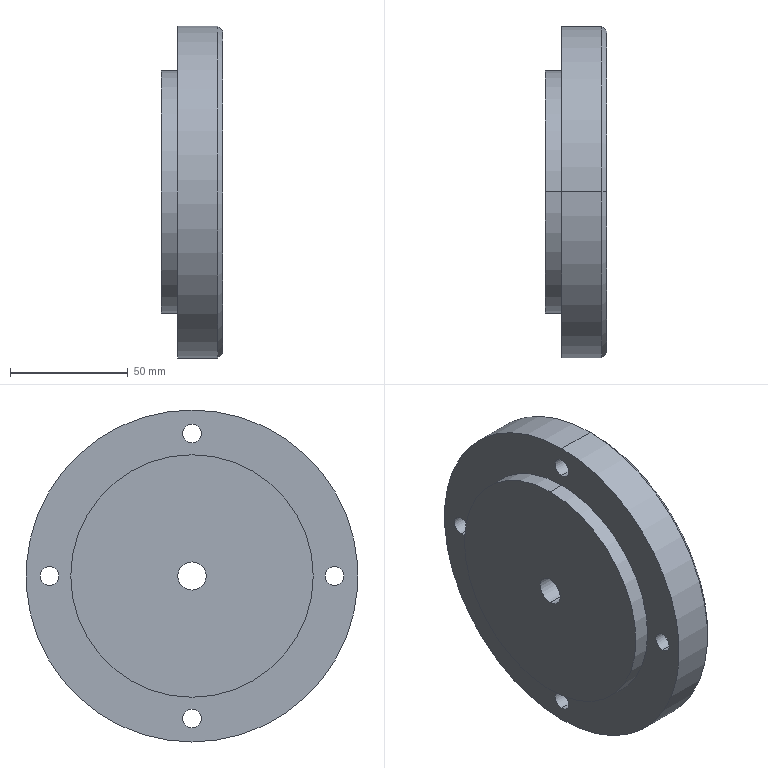Part | SolidWorks | features ICE 2, Chamfer 1, Revolution 1 | 1 solid | 34 faces | box 26 x 141 x 141 mm | volume 338840 mm3 | cylinder 22 | plane 8 | cone 4 | commonest cylinder face diameters 8 x8 14 x8 12 x2 103 x2 141 x2
STEP:
#1=CARTESIAN_POINT('',(-8.742,-60.5,7.));
#2=VERTEX_POINT('',#1);
#3=CARTESIAN_POINT('',(-8.742,-60.5,-7.));
#4=VERTEX_POINT('',#3);
#5=CARTESIAN_POINT('',(-8.742,-60.5,0.));
#6=DIRECTION('',(1.,0.,0.));
#7=DIRECTION('',(0.,0.,-1.));
#8=AXIS2_PLACEMENT_3D('',#5,#6,#7);
#9=CIRCLE('',#8,7.);
#10=EDGE_CURVE('',#2,#4,#9,.T.);
#11=ORIENTED_EDGE('',*,*,#10,.F.);
#12=CARTESIAN_POINT('',(-2.742,-60.5,7.));
#13=VERTEX_POINT('',#12);
#14=CARTESIAN_POINT('',(-8.742,-60.5,7.));
#15=DIRECTION('',(1.,0.,0.));
#16=VECTOR('',#15,1000.);
#17=LINE('',#14,#16);
#18=EDGE_CURVE('',#2,#13,#17,.T.);
#19=ORIENTED_EDGE('',*,*,#18,.T.);
#20=CARTESIAN_POINT('',(-2.742,-60.5,-7.));
#21=VERTEX_POINT('',#20);
#22=CARTESIAN_POINT('',(-2.742,-60.5,0.));
#23=DIRECTION('',(1.,0.,0.));
#24=DIRECTION('',(0.,0.,-1.));
#25=AXIS2_PLACEMENT_3D('',#22,#23,#24);
#26=CIRCLE('',#25,7.);
#27=EDGE_CURVE('',#13,#21,#26,.T.);
#28=ORIENTED_EDGE('',*,*,#27,.T.);
#29=CARTESIAN_POINT('',(-8.742,-60.5,-7.));
#30=DIRECTION('',(1.,0.,0.));
#31=VECTOR('',#30,1000.);
#32=LINE('',#29,#31);
#33=EDGE_CURVE('',#4,#21,#32,.T.);
#34=ORIENTED_EDGE('',*,*,#33,.F.);
#35=EDGE_LOOP('',(#11,#19,#28,#34));
#36=FACE_OUTER_BOUND('',#35,.T.);
#37=CARTESIAN_POINT('',(-8.742,-60.5,0.));
#38=DIRECTION('',(1.,0.,0.));
#39=DIRECTION('',(0.,0.,-1.));
#40=AXIS2_PLACEMENT_3D('',#37,#38,#39);
#41=CYLINDRICAL_SURFACE('',#40,7.);
#42=ADVANCED_FACE('',(#36),#41,.F.);
#43=CARTESIAN_POINT('',(-8.742,0.,-53.5));
#44=VERTEX_POINT('',#43);
#45=CARTESIAN_POINT('',(-8.742,0.,-67.5));
#46=VERTEX_POINT('',#45);
#47=CARTESIAN_POINT('',(-8.742,0.,-60.5));
#48=DIRECTION('',(1.,0.,0.));
#49=DIRECTION('',(0.,0.,-1.));
#50=AXIS2_PLACEMENT_3D('',#47,#48,#49);
#51=CIRCLE('',#50,7.);
#52=EDGE_CURVE('',#44,#46,#51,.T.);
#53=ORIENTED_EDGE('',*,*,#52,.F.);
#54=CARTESIAN_POINT('',(-2.742,0.,-53.5));
#55=VERTEX_POINT('',#54);
#56=CARTESIAN_POINT('',(-8.742,0.,-53.5));
#57=DIRECTION('',(1.,0.,0.));
#58=VECTOR('',#57,1000.);
#59=LINE('',#56,#58);
#60=EDGE_CURVE('',#44,#55,#59,.T.);
#61=ORIENTED_EDGE('',*,*,#60,.T.);
#62=CARTESIAN_POINT('',(-2.742,0.,-67.5));
#63=VERTEX_POINT('',#62);
#64=CARTESIAN_POINT('',(-2.742,0.,-60.5));
#65=DIRECTION('',(1.,0.,0.));
#66=DIRECTION('',(0.,0.,-1.));
#67=AXIS2_PLACEMENT_3D('',#64,#65,#66);
#68=CIRCLE('',#67,7.);
#69=EDGE_CURVE('',#55,#63,#68,.T.);
#70=ORIENTED_EDGE('',*,*,#69,.T.);
#71=CARTESIAN_POINT('',(-8.742,0.,-67.5));
#72=DIRECTION('',(1.,0.,0.));
#73=VECTOR('',#72,1000.);
#74=LINE('',#71,#73);
#75=EDGE_CURVE('',#46,#63,#74,.T.);
#76=ORIENTED_EDGE('',*,*,#75,.F.);
#77=EDGE_LOOP('',(#53,#61,#70,#76));
#78=FACE_OUTER_BOUND('',#77,.T.);
#79=CARTESIAN_POINT('',(-8.742,0.,-60.5));
#80=DIRECTION('',(1.,0.,0.));
#81=DIRECTION('',(0.,0.,-1.));
#82=AXIS2_PLACEMENT_3D('',#79,#80,#81);
#83=CYLINDRICAL_SURFACE('',#82,7.);
#84=ADVANCED_FACE('',(#78),#83,.F.);
#85=CARTESIAN_POINT('',(-8.742,60.5,7.));
#86=VERTEX_POINT('',#85);
#87=CARTESIAN_POINT('',(-8.742,60.5,-7.));
#88=VERTEX_POINT('',#87);
#89=CARTESIAN_POINT('',(-8.742,60.5,0.));
#90=DIRECTION('',(1.,0.,0.));
#91=DIRECTION('',(0.,0.,-1.));
#92=AXIS2_PLACEMENT_3D('',#89,#90,#91);
#93=CIRCLE('',#92,7.);
#94=EDGE_CURVE('',#86,#88,#93,.T.);
#95=ORIENTED_EDGE('',*,*,#94,.F.);
#96=CARTESIAN_POINT('',(-2.742,60.5,7.));
#97=VERTEX_POINT('',#96);
#98=CARTESIAN_POINT('',(-8.742,60.5,7.));
#99=DIRECTION('',(1.,0.,0.));
#100=VECTOR('',#99,1000.);
#101=LINE('',#98,#100);
#102=EDGE_CURVE('',#86,#97,#101,.T.);
#103=ORIENTED_EDGE('',*,*,#102,.T.);
#104=CARTESIAN_POINT('',(-2.742,60.5,-7.));
#105=VERTEX_POINT('',#104);
#106=CARTESIAN_POINT('',(-2.742,60.5,0.));
#107=DIRECTION('',(1.,0.,0.));
#108=DIRECTION('',(0.,0.,-1.));
#109=AXIS2_PLACEMENT_3D('',#106,#107,#108);
#110=CIRCLE('',#109,7.);
#111=EDGE_CURVE('',#97,#105,#110,.T.);
#112=ORIENTED_EDGE('',*,*,#111,.T.);
#113=CARTESIAN_POINT('',(-8.742,60.5,-7.));
#114=DIRECTION('',(1.,0.,0.));
#115=VECTOR('',#114,1000.);
#116=LINE('',#113,#115);
#117=EDGE_CURVE('',#88,#105,#116,.T.);
#118=ORIENTED_EDGE('',*,*,#117,.F.);
#119=EDGE_LOOP('',(#95,#103,#112,#118));
#120=FACE_OUTER_BOUND('',#119,.T.);
#121=CARTESIAN_POINT('',(-8.742,60.5,0.));
#122=DIRECTION('',(1.,0.,0.));
#123=DIRECTION('',(0.,0.,-1.));
#124=AXIS2_PLACEMENT_3D('',#121,#122,#123);
#125=CYLINDRICAL_SURFACE('',#124,7.);
#126=ADVANCED_FACE('',(#120),#125,.F.);
#127=CARTESIAN_POINT('',(-8.742,0.,67.5));
#128=VERTEX_POINT('',#127);
#129=CARTESIAN_POINT('',(-8.742,0.,53.5));
#130=VERTEX_POINT('',#129);
#131=CARTESIAN_POINT('',(-8.742,0.,60.5));
#132=DIRECTION('',(1.,0.,0.));
#133=DIRECTION('',(0.,0.,-1.));
#134=AXIS2_PLACEMENT_3D('',#131,#132,#133);
#135=CIRCLE('',#134,7.);
#136=EDGE_CURVE('',#128,#130,#135,.T.);
#137=ORIENTED_EDGE('',*,*,#136,.F.);
#138=CARTESIAN_POINT('',(-2.742,0.,67.5));
#139=VERTEX_POINT('',#138);
#140=CARTESIAN_POINT('',(-8.742,0.,67.5));
#141=DIRECTION('',(1.,0.,0.));
#142=VECTOR('',#141,1000.);
#143=LINE('',#140,#142);
#144=EDGE_CURVE('',#128,#139,#143,.T.);
#145=ORIENTED_EDGE('',*,*,#144,.T.);
#146=CARTESIAN_POINT('',(-2.742,0.,53.5));
#147=VERTEX_POINT('',#146);
#148=CARTESIAN_POINT('',(-2.742,0.,60.5));
#149=DIRECTION('',(1.,0.,0.));
#150=DIRECTION('',(0.,0.,-1.));
#151=AXIS2_PLACEMENT_3D('',#148,#149,#150);
#152=CIRCLE('',#151,7.);
#153=EDGE_CURVE('',#139,#147,#152,.T.);
#154=ORIENTED_EDGE('',*,*,#153,.T.);
#155=CARTESIAN_POINT('',(-8.742,0.,53.5));
#156=DIRECTION('',(1.,0.,0.));
#157=VECTOR('',#156,1000.);
#158=LINE('',#155,#157);
#159=EDGE_CURVE('',#130,#147,#158,.T.);
#160=ORIENTED_EDGE('',*,*,#159,.F.);
#161=EDGE_LOOP('',(#137,#145,#154,#160));
#162=FACE_OUTER_BOUND('',#161,.T.);
#163=CARTESIAN_POINT('',(-8.742,0.,60.5));
#164=DIRECTION('',(1.,0.,0.));
#165=DIRECTION('',(0.,0.,-1.));
#166=AXIS2_PLACEMENT_3D('',#163,#164,#165);
#167=CYLINDRICAL_SURFACE('',#166,7.);
#168=ADVANCED_FACE('',(#162),#167,.F.);
#169=CARTESIAN_POINT('',(-2.742,0.,-68.5));
#170=VERTEX_POINT('',#169);
#171=CARTESIAN_POINT('',(-2.742,0.,68.5));
#172=VERTEX_POINT('',#171);
#173=CARTESIAN_POINT('',(-2.742,0.,0.));
#174=DIRECTION('',(1.,0.,0.));
#175=DIRECTION('',(0.,0.,1.));
#176=AXIS2_PLACEMENT_3D('',#173,#174,#175);
#177=CIRCLE('',#176,68.5);
#178=EDGE_CURVE('',#170,#172,#177,.T.);
#179=ORIENTED_EDGE('',*,*,#178,.F.);
#180=CARTESIAN_POINT('',(-4.742,0.,-70.5));
#181=VERTEX_POINT('',#180);
#182=CARTESIAN_POINT('',(-4.742,0.,-70.5));
#183=DIRECTION('',(-0.7071,0.,-0.7071));
#184=VECTOR('',#183,1000.);
#185=LINE('',#182,#184);
#186=EDGE_CURVE('',#170,#181,#185,.T.);
#187=ORIENTED_EDGE('',*,*,#186,.T.);
#188=CARTESIAN_POINT('',(-4.742,0.,70.5));
#189=VERTEX_POINT('',#188);
#190=CARTESIAN_POINT('',(-4.742,0.,0.));
#191=DIRECTION('',(-1.,0.,0.));
#192=DIRECTION('',(0.,0.,1.));
#193=AXIS2_PLACEMENT_3D('',#190,#191,#192);
#194=CIRCLE('',#193,70.5);
#195=EDGE_CURVE('',#189,#181,#194,.T.);
#196=ORIENTED_EDGE('',*,*,#195,.F.);
#197=CARTESIAN_POINT('',(-4.742,0.,70.5));
#198=DIRECTION('',(-0.7071,0.,0.7071));
#199=VECTOR('',#198,1000.);
#200=LINE('',#197,#199);
#201=EDGE_CURVE('',#172,#189,#200,.T.);
#202=ORIENTED_EDGE('',*,*,#201,.F.);
#203=EDGE_LOOP('',(#179,#187,#196,#202));
#204=FACE_OUTER_BOUND('',#203,.T.);
#205=CARTESIAN_POINT('',(-4.742,0.,0.));
#206=DIRECTION('',(-1.,0.,0.));
#207=DIRECTION('',(0.,0.,1.));
#208=AXIS2_PLACEMENT_3D('',#205,#206,#207);
#209=CONICAL_SURFACE('',#208,70.5,0.7854);
#210=ADVANCED_FACE('',(#204),#209,.T.);
#211=CARTESIAN_POINT('',(-10.031,0.,-14.747));
#212=VERTEX_POINT('',#211);
#213=CARTESIAN_POINT('',(-10.031,0.,14.747));
#214=VERTEX_POINT('',#213);
#215=CARTESIAN_POINT('',(-10.031,0.,0.));
#216=DIRECTION('',(-1.,0.,0.));
#217=DIRECTION('',(0.,0.,1.));
#218=AXIS2_PLACEMENT_3D('',#215,#216,#217);
#219=CIRCLE('',#218,14.747);
#220=EDGE_CURVE('',#212,#214,#219,.T.);
#221=ORIENTED_EDGE('',*,*,#220,.T.);
#222=CARTESIAN_POINT('',(-2.742,0.,19.746));
#223=VERTEX_POINT('',#222);
#224=CARTESIAN_POINT('',(-10.031,0.,14.747));
#225=DIRECTION('',(0.8247,0.,0.5655));
#226=VECTOR('',#225,1000.);
#227=LINE('',#224,#226);
#228=EDGE_CURVE('',#214,#223,#227,.T.);
#229=ORIENTED_EDGE('',*,*,#228,.T.);
#230=CARTESIAN_POINT('',(-2.742,0.,-19.746));
#231=VERTEX_POINT('',#230);
#232=CARTESIAN_POINT('',(-2.742,0.,0.));
#233=DIRECTION('',(-1.,0.,0.));
#234=DIRECTION('',(0.,0.,1.));
#235=AXIS2_PLACEMENT_3D('',#232,#233,#234);
#236=CIRCLE('',#235,19.746);
#237=EDGE_CURVE('',#231,#223,#236,.T.);
#238=ORIENTED_EDGE('',*,*,#237,.F.);
#239=CARTESIAN_POINT('',(-10.031,0.,-14.747));
#240=DIRECTION('',(0.8247,0.,-0.5655));
#241=VECTOR('',#240,1000.);
#242=LINE('',#239,#241);
#243=EDGE_CURVE('',#212,#231,#242,.T.);
#244=ORIENTED_EDGE('',*,*,#243,.F.);
#245=EDGE_LOOP('',(#221,#229,#238,#244));
#246=FACE_OUTER_BOUND('',#245,.T.);
#247=CARTESIAN_POINT('',(-10.031,0.,0.));
#248=DIRECTION('',(1.,0.,0.));
#249=DIRECTION('',(0.,0.,-1.));
#250=AXIS2_PLACEMENT_3D('',#247,#248,#249);
#251=CONICAL_SURFACE('',#250,14.747,0.6011);
#252=ADVANCED_FACE('',(#246),#251,.F.);
#253=ORIENTED_EDGE('',*,*,#195,.T.);
#254=CARTESIAN_POINT('',(-21.742,0.,-70.5));
#255=VERTEX_POINT('',#254);
#256=CARTESIAN_POINT('',(-75.394,0.,-70.5));
#257=DIRECTION('',(-1.,0.,0.));
#258=VECTOR('',#257,1000.);
#259=LINE('',#256,#258);
#260=EDGE_CURVE('',#181,#255,#259,.T.);
#261=ORIENTED_EDGE('',*,*,#260,.T.);
#262=CARTESIAN_POINT('',(-21.742,0.,70.5));
#263=VERTEX_POINT('',#262);
#264=CARTESIAN_POINT('',(-21.742,0.,0.));
#265=DIRECTION('',(-1.,0.,0.));
#266=DIRECTION('',(0.,0.,1.));
#267=AXIS2_PLACEMENT_3D('',#264,#265,#266);
#268=CIRCLE('',#267,70.5);
#269=EDGE_CURVE('',#263,#255,#268,.T.);
#270=ORIENTED_EDGE('',*,*,#269,.F.);
#271=CARTESIAN_POINT('',(-75.394,0.,70.5));
#272=DIRECTION('',(-1.,0.,0.));
#273=VECTOR('',#272,1000.);
#274=LINE('',#271,#273);
#275=EDGE_CURVE('',#189,#263,#274,.T.);
#276=ORIENTED_EDGE('',*,*,#275,.F.);
#277=EDGE_LOOP('',(#253,#261,#270,#276));
#278=FACE_OUTER_BOUND('',#277,.T.);
#279=CARTESIAN_POINT('',(-75.394,0.,0.));
#280=DIRECTION('',(-1.,0.,0.));
#281=DIRECTION('',(0.,0.,1.));
#282=AXIS2_PLACEMENT_3D('',#279,#280,#281);
#283=CYLINDRICAL_SURFACE('',#282,70.5);
#284=ADVANCED_FACE('',(#278),#283,.T.);
#285=CARTESIAN_POINT('',(-21.742,0.,51.5));
#286=VERTEX_POINT('',#285);
#287=CARTESIAN_POINT('',(-21.742,0.,-51.5));
#288=VERTEX_POINT('',#287);
#289=CARTESIAN_POINT('',(-21.742,0.,0.));
#290=DIRECTION('',(-1.,0.,0.));
#291=DIRECTION('',(0.,0.,1.));
#292=AXIS2_PLACEMENT_3D('',#289,#290,#291);
#293=CIRCLE('',#292,51.5);
#294=EDGE_CURVE('',#286,#288,#293,.T.);
#295=ORIENTED_EDGE('',*,*,#294,.T.);
#296=CARTESIAN_POINT('',(-28.742,0.,-51.5));
#297=VERTEX_POINT('',#296);
#298=CARTESIAN_POINT('',(-75.394,0.,-51.5));
#299=DIRECTION('',(-1.,0.,0.));
#300=VECTOR('',#299,1000.);
#301=LINE('',#298,#300);
#302=EDGE_CURVE('',#288,#297,#301,.T.);
#303=ORIENTED_EDGE('',*,*,#302,.T.);
#304=CARTESIAN_POINT('',(-28.742,0.,51.5));
#305=VERTEX_POINT('',#304);
#306=CARTESIAN_POINT('',(-28.742,0.,0.));
#307=DIRECTION('',(-1.,0.,0.));
#308=DIRECTION('',(0.,0.,1.));
#309=AXIS2_PLACEMENT_3D('',#306,#307,#308);
#310=CIRCLE('',#309,51.5);
#311=EDGE_CURVE('',#305,#297,#310,.T.);
#312=ORIENTED_EDGE('',*,*,#311,.F.);
#313=CARTESIAN_POINT('',(-75.394,0.,51.5));
#314=DIRECTION('',(-1.,0.,0.));
#315=VECTOR('',#314,1000.);
#316=LINE('',#313,#315);
#317=EDGE_CURVE('',#286,#305,#316,.T.);
#318=ORIENTED_EDGE('',*,*,#317,.F.);
#319=EDGE_LOOP('',(#295,#303,#312,#318));
#320=FACE_OUTER_BOUND('',#319,.T.);
#321=CARTESIAN_POINT('',(-75.394,0.,0.));
#322=DIRECTION('',(-1.,0.,0.));
#323=DIRECTION('',(0.,0.,1.));
#324=AXIS2_PLACEMENT_3D('',#321,#322,#323);
#325=CYLINDRICAL_SURFACE('',#324,51.5);
#326=ADVANCED_FACE('',(#320),#325,.T.);
#327=CARTESIAN_POINT('',(-10.031,0.,-6.));
#328=VERTEX_POINT('',#327);
#329=CARTESIAN_POINT('',(-10.031,0.,6.));
#330=VERTEX_POINT('',#329);
#331=CARTESIAN_POINT('',(-10.031,0.,0.));
#332=DIRECTION('',(-1.,0.,0.));
#333=DIRECTION('',(0.,0.,1.));
#334=AXIS2_PLACEMENT_3D('',#331,#332,#333);
#335=CIRCLE('',#334,6.);
#336=EDGE_CURVE('',#328,#330,#335,.T.);
#337=ORIENTED_EDGE('',*,*,#336,.F.);
#338=CARTESIAN_POINT('',(-28.742,0.,-6.));
#339=VERTEX_POINT('',#338);
#340=CARTESIAN_POINT('',(-75.394,0.,-6.));
#341=DIRECTION('',(-1.,0.,0.));
#342=VECTOR('',#341,1000.);
#343=LINE('',#340,#342);
#344=EDGE_CURVE('',#328,#339,#343,.T.);
#345=ORIENTED_EDGE('',*,*,#344,.T.);
#346=CARTESIAN_POINT('',(-28.742,0.,6.));
#347=VERTEX_POINT('',#346);
#348=CARTESIAN_POINT('',(-28.742,0.,0.));
#349=DIRECTION('',(-1.,0.,0.));
#350=DIRECTION('',(0.,0.,1.));
#351=AXIS2_PLACEMENT_3D('',#348,#349,#350);
#352=CIRCLE('',#351,6.);
#353=EDGE_CURVE('',#339,#347,#352,.T.);
#354=ORIENTED_EDGE('',*,*,#353,.T.);
#355=CARTESIAN_POINT('',(-75.394,0.,6.));
#356=DIRECTION('',(-1.,0.,0.));
#357=VECTOR('',#356,1000.);
#358=LINE('',#355,#357);
#359=EDGE_CURVE('',#330,#347,#358,.T.);
#360=ORIENTED_EDGE('',*,*,#359,.F.);
#361=EDGE_LOOP('',(#337,#345,#354,#360));
#362=FACE_OUTER_BOUND('',#361,.T.);
#363=CARTESIAN_POINT('',(-75.394,0.,0.));
#364=DIRECTION('',(-1.,0.,0.));
#365=DIRECTION('',(0.,0.,1.));
#366=AXIS2_PLACEMENT_3D('',#363,#364,#365);
#367=CYLINDRICAL_SURFACE('',#366,6.);
#368=ADVANCED_FACE('',(#362),#367,.F.);
#369=CARTESIAN_POINT('',(-21.742,0.,64.5));
#370=VERTEX_POINT('',#369);
#371=CARTESIAN_POINT('',(-21.742,0.,56.5));
#372=VERTEX_POINT('',#371);
#373=CARTESIAN_POINT('',(-21.742,0.,60.5));
#374=DIRECTION('',(1.,0.,0.));
#375=DIRECTION('',(0.,0.,-1.));
#376=AXIS2_PLACEMENT_3D('',#373,#374,#375);
#377=CIRCLE('',#376,4.);
#378=EDGE_CURVE('',#370,#372,#377,.T.);
#379=ORIENTED_EDGE('',*,*,#378,.F.);
#380=CARTESIAN_POINT('',(-8.742,0.,64.5));
#381=VERTEX_POINT('',#380);
#382=CARTESIAN_POINT('',(-51.742,0.,64.5));
#383=DIRECTION('',(1.,0.,0.));
#384=VECTOR('',#383,1000.);
#385=LINE('',#382,#384);
#386=EDGE_CURVE('',#370,#381,#385,.T.);
#387=ORIENTED_EDGE('',*,*,#386,.T.);
#388=CARTESIAN_POINT('',(-8.742,0.,56.5));
#389=VERTEX_POINT('',#388);
#390=CARTESIAN_POINT('',(-8.742,0.,60.5));
#391=DIRECTION('',(-1.,0.,0.));
#392=DIRECTION('',(0.,0.,-1.));
#393=AXIS2_PLACEMENT_3D('',#390,#391,#392);
#394=CIRCLE('',#393,4.);
#395=EDGE_CURVE('',#389,#381,#394,.T.);
#396=ORIENTED_EDGE('',*,*,#395,.F.);
#397=CARTESIAN_POINT('',(-51.742,0.,56.5));
#398=DIRECTION('',(1.,0.,0.));
#399=VECTOR('',#398,1000.);
#400=LINE('',#397,#399);
#401=EDGE_CURVE('',#372,#389,#400,.T.);
#402=ORIENTED_EDGE('',*,*,#401,.F.);
#403=EDGE_LOOP('',(#379,#387,#396,#402));
#404=FACE_OUTER_BOUND('',#403,.T.);
#405=CARTESIAN_POINT('',(-51.742,0.,60.5));
#406=DIRECTION('',(1.,0.,0.));
#407=DIRECTION('',(0.,0.,-1.));
#408=AXIS2_PLACEMENT_3D('',#405,#406,#407);
#409=CYLINDRICAL_SURFACE('',#408,4.);
#410=ADVANCED_FACE('',(#404),#409,.F.);
#411=CARTESIAN_POINT('',(-21.742,60.5,4.));
#412=VERTEX_POINT('',#411);
#413=CARTESIAN_POINT('',(-21.742,60.5,-4.));
#414=VERTEX_POINT('',#413);
#415=CARTESIAN_POINT('',(-21.742,60.5,0.));
#416=DIRECTION('',(1.,0.,0.));
#417=DIRECTION('',(0.,0.,-1.));
#418=AXIS2_PLACEMENT_3D('',#415,#416,#417);
#419=CIRCLE('',#418,4.);
#420=EDGE_CURVE('',#412,#414,#419,.T.);
#421=ORIENTED_EDGE('',*,*,#420,.F.);
#422=CARTESIAN_POINT('',(-8.742,60.5,4.));
#423=VERTEX_POINT('',#422);
#424=CARTESIAN_POINT('',(-51.742,60.5,4.));
#425=DIRECTION('',(1.,0.,0.));
#426=VECTOR('',#425,1000.);
#427=LINE('',#424,#426);
#428=EDGE_CURVE('',#412,#423,#427,.T.);
#429=ORIENTED_EDGE('',*,*,#428,.T.);
#430=CARTESIAN_POINT('',(-8.742,60.5,-4.));
#431=VERTEX_POINT('',#430);
#432=CARTESIAN_POINT('',(-8.742,60.5,0.));
#433=DIRECTION('',(-1.,0.,0.));
#434=DIRECTION('',(0.,0.,-1.));
#435=AXIS2_PLACEMENT_3D('',#432,#433,#434);
#436=CIRCLE('',#435,4.);
#437=EDGE_CURVE('',#431,#423,#436,.T.);
#438=ORIENTED_EDGE('',*,*,#437,.F.);
#439=CARTESIAN_POINT('',(-51.742,60.5,-4.));
#440=DIRECTION('',(1.,0.,0.));
#441=VECTOR('',#440,1000.);
#442=LINE('',#439,#441);
#443=EDGE_CURVE('',#414,#431,#442,.T.);
#444=ORIENTED_EDGE('',*,*,#443,.F.);
#445=EDGE_LOOP('',(#421,#429,#438,#444));
#446=FACE_OUTER_BOUND('',#445,.T.);
#447=CARTESIAN_POINT('',(-51.742,60.5,0.));
#448=DIRECTION('',(1.,0.,0.));
#449=DIRECTION('',(0.,0.,-1.));
#450=AXIS2_PLACEMENT_3D('',#447,#448,#449);
#451=CYLINDRICAL_SURFACE('',#450,4.);
#452=ADVANCED_FACE('',(#446),#451,.F.);
#453=CARTESIAN_POINT('',(-21.742,0.,-56.5));
#454=VERTEX_POINT('',#453);
#455=CARTESIAN_POINT('',(-21.742,0.,-64.5));
#456=VERTEX_POINT('',#455);
#457=CARTESIAN_POINT('',(-21.742,0.,-60.5));
#458=DIRECTION('',(1.,0.,0.));
#459=DIRECTION('',(0.,0.,-1.));
#460=AXIS2_PLACEMENT_3D('',#457,#458,#459);
#461=CIRCLE('',#460,4.);
#462=EDGE_CURVE('',#454,#456,#461,.T.);
#463=ORIENTED_EDGE('',*,*,#462,.F.);
#464=CARTESIAN_POINT('',(-8.742,0.,-56.5));
#465=VERTEX_POINT('',#464);
#466=CARTESIAN_POINT('',(-51.742,0.,-56.5));
#467=DIRECTION('',(1.,0.,0.));
#468=VECTOR('',#467,1000.);
#469=LINE('',#466,#468);
#470=EDGE_CURVE('',#454,#465,#469,.T.);
#471=ORIENTED_EDGE('',*,*,#470,.T.);
#472=CARTESIAN_POINT('',(-8.742,0.,-64.5));
#473=VERTEX_POINT('',#472);
#474=CARTESIAN_POINT('',(-8.742,0.,-60.5));
#475=DIRECTION('',(-1.,0.,0.));
#476=DIRECTION('',(0.,0.,-1.));
#477=AXIS2_PLACEMENT_3D('',#474,#475,#476);
#478=CIRCLE('',#477,4.);
#479=EDGE_CURVE('',#473,#465,#478,.T.);
#480=ORIENTED_EDGE('',*,*,#479,.F.);
#481=CARTESIAN_POINT('',(-51.742,0.,-64.5));
#482=DIRECTION('',(1.,0.,0.));
#483=VECTOR('',#482,1000.);
#484=LINE('',#481,#483);
#485=EDGE_CURVE('',#456,#473,#484,.T.);
#486=ORIENTED_EDGE('',*,*,#485,.F.);
#487=EDGE_LOOP('',(#463,#471,#480,#486));
#488=FACE_OUTER_BOUND('',#487,.T.);
#489=CARTESIAN_POINT('',(-51.742,0.,-60.5));
#490=DIRECTION('',(1.,0.,0.));
#491=DIRECTION('',(0.,0.,-1.));
#492=AXIS2_PLACEMENT_3D('',#489,#490,#491);
#493=CYLINDRICAL_SURFACE('',#492,4.);
#494=ADVANCED_FACE('',(#488),#493,.F.);
#495=CARTESIAN_POINT('',(-21.742,-60.5,4.));
#496=VERTEX_POINT('',#495);
#497=CARTESIAN_POINT('',(-21.742,-60.5,-4.));
#498=VERTEX_POINT('',#497);
#499=CARTESIAN_POINT('',(-21.742,-60.5,0.));
#500=DIRECTION('',(1.,0.,0.));
#501=DIRECTION('',(0.,0.,-1.));
#502=AXIS2_PLACEMENT_3D('',#499,#500,#501);
#503=CIRCLE('',#502,4.);
#504=EDGE_CURVE('',#496,#498,#503,.T.);
#505=ORIENTED_EDGE('',*,*,#504,.F.);
#506=CARTESIAN_POINT('',(-8.742,-60.5,4.));
#507=VERTEX_POINT('',#506);
#508=CARTESIAN_POINT('',(-51.742,-60.5,4.));
#509=DIRECTION('',(1.,0.,0.));
#510=VECTOR('',#509,1000.);
#511=LINE('',#508,#510);
#512=EDGE_CURVE('',#496,#507,#511,.T.);
#513=ORIENTED_EDGE('',*,*,#512,.T.);
#514=CARTESIAN_POINT('',(-8.742,-60.5,-4.));
#515=VERTEX_POINT('',#514);
#516=CARTESIAN_POINT('',(-8.742,-60.5,0.));
#517=DIRECTION('',(-1.,0.,0.));
#518=DIRECTION('',(0.,0.,-1.));
#519=AXIS2_PLACEMENT_3D('',#516,#517,#518);
#520=CIRCLE('',#519,4.);
#521=EDGE_CURVE('',#515,#507,#520,.T.);
#522=ORIENTED_EDGE('',*,*,#521,.F.);
#523=CARTESIAN_POINT('',(-51.742,-60.5,-4.));
#524=DIRECTION('',(1.,0.,0.));
#525=VECTOR('',#524,1000.);
#526=LINE('',#523,#525);
#527=EDGE_CURVE('',#498,#515,#526,.T.);
#528=ORIENTED_EDGE('',*,*,#527,.F.);
#529=EDGE_LOOP('',(#505,#513,#522,#528));
#530=FACE_OUTER_BOUND('',#529,.T.);
#531=CARTESIAN_POINT('',(-51.742,-60.5,0.));
#532=DIRECTION('',(1.,0.,0.));
#533=DIRECTION('',(0.,0.,-1.));
#534=AXIS2_PLACEMENT_3D('',#531,#532,#533);
#535=CYLINDRICAL_SURFACE('',#534,4.);
#536=ADVANCED_FACE('',(#530),#535,.F.);
#537=ORIENTED_EDGE('',*,*,#512,.F.);
#538=CARTESIAN_POINT('',(-21.742,-60.5,0.));
#539=DIRECTION('',(1.,0.,0.));
#540=DIRECTION('',(0.,0.,-1.));
#541=AXIS2_PLACEMENT_3D('',#538,#539,#540);
#542=CIRCLE('',#541,4.);
#543=EDGE_CURVE('',#498,#496,#542,.T.);
#544=ORIENTED_EDGE('',*,*,#543,.F.);
#545=ORIENTED_EDGE('',*,*,#527,.T.);
#546=CARTESIAN_POINT('',(-8.742,-60.5,0.));
#547=DIRECTION('',(-1.,0.,0.));
#548=DIRECTION('',(0.,0.,-1.));
#549=AXIS2_PLACEMENT_3D('',#546,#547,#548);
#550=CIRCLE('',#549,4.);
#551=EDGE_CURVE('',#507,#515,#550,.T.);
#552=ORIENTED_EDGE('',*,*,#551,.F.);
#553=EDGE_LOOP('',(#537,#544,#545,#552));
#554=FACE_OUTER_BOUND('',#553,.T.);
#555=CARTESIAN_POINT('',(-51.742,-60.5,0.));
#556=DIRECTION('',(1.,0.,0.));
#557=DIRECTION('',(0.,0.,-1.));
#558=AXIS2_PLACEMENT_3D('',#555,#556,#557);
#559=CYLINDRICAL_SURFACE('',#558,4.);
#560=ADVANCED_FACE('',(#554),#559,.F.);
#561=ORIENTED_EDGE('',*,*,#470,.F.);
#562=CARTESIAN_POINT('',(-21.742,0.,-60.5));
#563=DIRECTION('',(1.,0.,0.));
#564=DIRECTION('',(0.,0.,-1.));
#565=AXIS2_PLACEMENT_3D('',#562,#563,#564);
#566=CIRCLE('',#565,4.);
#567=EDGE_CURVE('',#456,#454,#566,.T.);
#568=ORIENTED_EDGE('',*,*,#567,.F.);
#569=ORIENTED_EDGE('',*,*,#485,.T.);
#570=CARTESIAN_POINT('',(-8.742,0.,-60.5));
#571=DIRECTION('',(-1.,0.,0.));
#572=DIRECTION('',(0.,0.,-1.));
#573=AXIS2_PLACEMENT_3D('',#570,#571,#572);
#574=CIRCLE('',#573,4.);
#575=EDGE_CURVE('',#465,#473,#574,.T.);
#576=ORIENTED_EDGE('',*,*,#575,.F.);
#577=EDGE_LOOP('',(#561,#568,#569,#576));
#578=FACE_OUTER_BOUND('',#577,.T.);
#579=CARTESIAN_POINT('',(-51.742,0.,-60.5));
#580=DIRECTION('',(1.,0.,0.));
#581=DIRECTION('',(0.,0.,-1.));
#582=AXIS2_PLACEMENT_3D('',#579,#580,#581);
#583=CYLINDRICAL_SURFACE('',#582,4.);
#584=ADVANCED_FACE('',(#578),#583,.F.);
#585=ORIENTED_EDGE('',*,*,#428,.F.);
#586=CARTESIAN_POINT('',(-21.742,60.5,0.));
#587=DIRECTION('',(1.,0.,0.));
#588=DIRECTION('',(0.,0.,-1.));
#589=AXIS2_PLACEMENT_3D('',#586,#587,#588);
#590=CIRCLE('',#589,4.);
#591=EDGE_CURVE('',#414,#412,#590,.T.);
#592=ORIENTED_EDGE('',*,*,#591,.F.);
#593=ORIENTED_EDGE('',*,*,#443,.T.);
#594=CARTESIAN_POINT('',(-8.742,60.5,0.));
#595=DIRECTION('',(-1.,0.,0.));
#596=DIRECTION('',(0.,0.,-1.));
#597=AXIS2_PLACEMENT_3D('',#594,#595,#596);
#598=CIRCLE('',#597,4.);
#599=EDGE_CURVE('',#423,#431,#598,.T.);
#600=ORIENTED_EDGE('',*,*,#599,.F.);
#601=EDGE_LOOP('',(#585,#592,#593,#600));
#602=FACE_OUTER_BOUND('',#601,.T.);
#603=CARTESIAN_POINT('',(-51.742,60.5,0.));
#604=DIRECTION('',(1.,0.,0.));
#605=DIRECTION('',(0.,0.,-1.));
#606=AXIS2_PLACEMENT_3D('',#603,#604,#605);
#607=CYLINDRICAL_SURFACE('',#606,4.);
#608=ADVANCED_FACE('',(#602),#607,.F.);
#609=ORIENTED_EDGE('',*,*,#386,.F.);
#610=CARTESIAN_POINT('',(-21.742,0.,60.5));
#611=DIRECTION('',(1.,0.,0.));
#612=DIRECTION('',(0.,0.,-1.));
#613=AXIS2_PLACEMENT_3D('',#610,#611,#612);
#614=CIRCLE('',#613,4.);
#615=EDGE_CURVE('',#372,#370,#614,.T.);
#616=ORIENTED_EDGE('',*,*,#615,.F.);
#617=ORIENTED_EDGE('',*,*,#401,.T.);
#618=CARTESIAN_POINT('',(-8.742,0.,60.5));
#619=DIRECTION('',(-1.,0.,0.));
#620=DIRECTION('',(0.,0.,-1.));
#621=AXIS2_PLACEMENT_3D('',#618,#619,#620);
#622=CIRCLE('',#621,4.);
#623=EDGE_CURVE('',#381,#389,#622,.T.);
#624=ORIENTED_EDGE('',*,*,#623,.F.);
#625=EDGE_LOOP('',(#609,#616,#617,#624));
#626=FACE_OUTER_BOUND('',#625,.T.);
#627=CARTESIAN_POINT('',(-51.742,0.,60.5));
#628=DIRECTION('',(1.,0.,0.));
#629=DIRECTION('',(0.,0.,-1.));
#630=AXIS2_PLACEMENT_3D('',#627,#628,#629);
#631=CYLINDRICAL_SURFACE('',#630,4.);
#632=ADVANCED_FACE('',(#626),#631,.F.);
#633=ORIENTED_EDGE('',*,*,#344,.F.);
#634=CARTESIAN_POINT('',(-10.031,0.,0.));
#635=DIRECTION('',(-1.,0.,0.));
#636=DIRECTION('',(0.,0.,1.));
#637=AXIS2_PLACEMENT_3D('',#634,#635,#636);
#638=CIRCLE('',#637,6.);
#639=EDGE_CURVE('',#330,#328,#638,.T.);
#640=ORIENTED_EDGE('',*,*,#639,.F.);
#641=ORIENTED_EDGE('',*,*,#359,.T.);
#642=CARTESIAN_POINT('',(-28.742,0.,0.));
#643=DIRECTION('',(-1.,0.,0.));
#644=DIRECTION('',(0.,0.,1.));
#645=AXIS2_PLACEMENT_3D('',#642,#643,#644);
#646=CIRCLE('',#645,6.);
#647=EDGE_CURVE('',#347,#339,#646,.T.);
#648=ORIENTED_EDGE('',*,*,#647,.T.);
#649=EDGE_LOOP('',(#633,#640,#641,#648));
#650=FACE_OUTER_BOUND('',#649,.T.);
#651=CARTESIAN_POINT('',(-75.394,0.,0.));
#652=DIRECTION('',(-1.,0.,0.));
#653=DIRECTION('',(0.,0.,1.));
#654=AXIS2_PLACEMENT_3D('',#651,#652,#653);
#655=CYLINDRICAL_SURFACE('',#654,6.);
#656=ADVANCED_FACE('',(#650),#655,.F.);
#657=ORIENTED_EDGE('',*,*,#647,.F.);
#658=ORIENTED_EDGE('',*,*,#353,.F.);
#659=EDGE_LOOP('',(#657,#658));
#660=FACE_BOUND('',#659,.T.);
#661=ORIENTED_EDGE('',*,*,#311,.T.);
#662=CARTESIAN_POINT('',(-28.742,0.,0.));
#663=DIRECTION('',(-1.,0.,0.));
#664=DIRECTION('',(0.,0.,1.));
#665=AXIS2_PLACEMENT_3D('',#662,#663,#664);
#666=CIRCLE('',#665,51.5);
#667=EDGE_CURVE('',#297,#305,#666,.T.);
#668=ORIENTED_EDGE('',*,*,#667,.T.);
#669=EDGE_LOOP('',(#661,#668));
#670=FACE_OUTER_BOUND('',#669,.T.);
#671=CARTESIAN_POINT('',(-28.742,6.,0.));
#672=DIRECTION('',(1.,0.,0.));
#673=DIRECTION('',(0.,0.,-1.));
#674=AXIS2_PLACEMENT_3D('',#671,#672,#673);
#675=PLANE('',#674);
#676=ADVANCED_FACE('',(#660,#670),#675,.F.);
#677=ORIENTED_EDGE('',*,*,#302,.F.);
#678=CARTESIAN_POINT('',(-21.742,0.,0.));
#679=DIRECTION('',(-1.,0.,0.));
#680=DIRECTION('',(0.,0.,1.));
#681=AXIS2_PLACEMENT_3D('',#678,#679,#680);
#682=CIRCLE('',#681,51.5);
#683=EDGE_CURVE('',#288,#286,#682,.T.);
#684=ORIENTED_EDGE('',*,*,#683,.T.);
#685=ORIENTED_EDGE('',*,*,#317,.T.);
#686=ORIENTED_EDGE('',*,*,#667,.F.);
#687=EDGE_LOOP('',(#677,#684,#685,#686));
#688=FACE_OUTER_BOUND('',#687,.T.);
#689=CARTESIAN_POINT('',(-75.394,0.,0.));
#690=DIRECTION('',(-1.,0.,0.));
#691=DIRECTION('',(0.,0.,1.));
#692=AXIS2_PLACEMENT_3D('',#689,#690,#691);
#693=CYLINDRICAL_SURFACE('',#692,51.5);
#694=ADVANCED_FACE('',(#688),#693,.T.);
#695=ORIENTED_EDGE('',*,*,#615,.T.);
#696=ORIENTED_EDGE('',*,*,#378,.T.);
#697=EDGE_LOOP('',(#695,#696));
#698=FACE_BOUND('',#697,.T.);
#699=ORIENTED_EDGE('',*,*,#591,.T.);
#700=ORIENTED_EDGE('',*,*,#420,.T.);
#701=EDGE_LOOP('',(#699,#700));
#702=FACE_BOUND('',#701,.T.);
#703=ORIENTED_EDGE('',*,*,#567,.T.);
#704=ORIENTED_EDGE('',*,*,#462,.T.);
#705=EDGE_LOOP('',(#703,#704));
#706=FACE_BOUND('',#705,.T.);
#707=ORIENTED_EDGE('',*,*,#543,.T.);
#708=ORIENTED_EDGE('',*,*,#504,.T.);
#709=EDGE_LOOP('',(#707,#708));
#710=FACE_BOUND('',#709,.T.);
#711=ORIENTED_EDGE('',*,*,#294,.F.);
#712=ORIENTED_EDGE('',*,*,#683,.F.);
#713=EDGE_LOOP('',(#711,#712));
#714=FACE_BOUND('',#713,.T.);
#715=ORIENTED_EDGE('',*,*,#269,.T.);
#716=CARTESIAN_POINT('',(-21.742,0.,0.));
#717=DIRECTION('',(-1.,0.,0.));
#718=DIRECTION('',(0.,0.,1.));
#719=AXIS2_PLACEMENT_3D('',#716,#717,#718);
#720=CIRCLE('',#719,70.5);
#721=EDGE_CURVE('',#255,#263,#720,.T.);
#722=ORIENTED_EDGE('',*,*,#721,.T.);
#723=EDGE_LOOP('',(#715,#722));
#724=FACE_OUTER_BOUND('',#723,.T.);
#725=CARTESIAN_POINT('',(-21.742,51.5,0.));
#726=DIRECTION('',(1.,0.,0.));
#727=DIRECTION('',(0.,0.,-1.));
#728=AXIS2_PLACEMENT_3D('',#725,#726,#727);
#729=PLANE('',#728);
#730=ADVANCED_FACE('',(#698,#702,#706,#710,#714,#724),#729,.F.);
#731=ORIENTED_EDGE('',*,*,#260,.F.);
#732=CARTESIAN_POINT('',(-4.742,0.,0.));
#733=DIRECTION('',(-1.,0.,0.));
#734=DIRECTION('',(0.,0.,1.));
#735=AXIS2_PLACEMENT_3D('',#732,#733,#734);
#736=CIRCLE('',#735,70.5);
#737=EDGE_CURVE('',#181,#189,#736,.T.);
#738=ORIENTED_EDGE('',*,*,#737,.T.);
#739=ORIENTED_EDGE('',*,*,#275,.T.);
#740=ORIENTED_EDGE('',*,*,#721,.F.);
#741=EDGE_LOOP('',(#731,#738,#739,#740));
#742=FACE_OUTER_BOUND('',#741,.T.);
#743=CARTESIAN_POINT('',(-75.394,0.,0.));
#744=DIRECTION('',(-1.,0.,0.));
#745=DIRECTION('',(0.,0.,1.));
#746=AXIS2_PLACEMENT_3D('',#743,#744,#745);
#747=CYLINDRICAL_SURFACE('',#746,70.5);
#748=ADVANCED_FACE('',(#742),#747,.T.);
#749=CARTESIAN_POINT('',(-2.742,60.5,0.));
#750=DIRECTION('',(1.,0.,0.));
#751=DIRECTION('',(0.,0.,-1.));
#752=AXIS2_PLACEMENT_3D('',#749,#750,#751);
#753=CIRCLE('',#752,7.);
#754=EDGE_CURVE('',#105,#97,#753,.T.);
#755=ORIENTED_EDGE('',*,*,#754,.F.);
#756=ORIENTED_EDGE('',*,*,#111,.F.);
#757=EDGE_LOOP('',(#755,#756));
#758=FACE_BOUND('',#757,.T.);
#759=CARTESIAN_POINT('',(-2.742,0.,-60.5));
#760=DIRECTION('',(1.,0.,0.));
#761=DIRECTION('',(0.,0.,-1.));
#762=AXIS2_PLACEMENT_3D('',#759,#760,#761);
#763=CIRCLE('',#762,7.);
#764=EDGE_CURVE('',#63,#55,#763,.T.);
#765=ORIENTED_EDGE('',*,*,#764,.F.);
#766=ORIENTED_EDGE('',*,*,#69,.F.);
#767=EDGE_LOOP('',(#765,#766));
#768=FACE_BOUND('',#767,.T.);
#769=CARTESIAN_POINT('',(-2.742,-60.5,0.));
#770=DIRECTION('',(1.,0.,0.));
#771=DIRECTION('',(0.,0.,-1.));
#772=AXIS2_PLACEMENT_3D('',#769,#770,#771);
#773=CIRCLE('',#772,7.);
#774=EDGE_CURVE('',#21,#13,#773,.T.);
#775=ORIENTED_EDGE('',*,*,#774,.F.);
#776=ORIENTED_EDGE('',*,*,#27,.F.);
#777=EDGE_LOOP('',(#775,#776));
#778=FACE_BOUND('',#777,.T.);
#779=CARTESIAN_POINT('',(-2.742,0.,60.5));
#780=DIRECTION('',(1.,0.,0.));
#781=DIRECTION('',(0.,0.,-1.));
#782=AXIS2_PLACEMENT_3D('',#779,#780,#781);
#783=CIRCLE('',#782,7.);
#784=EDGE_CURVE('',#147,#139,#783,.T.);
#785=ORIENTED_EDGE('',*,*,#784,.F.);
#786=ORIENTED_EDGE('',*,*,#153,.F.);
#787=EDGE_LOOP('',(#785,#786));
#788=FACE_BOUND('',#787,.T.);
#789=CARTESIAN_POINT('',(-2.742,0.,0.));
#790=DIRECTION('',(1.,0.,0.));
#791=DIRECTION('',(0.,0.,1.));
#792=AXIS2_PLACEMENT_3D('',#789,#790,#791);
#793=CIRCLE('',#792,68.5);
#794=EDGE_CURVE('',#172,#170,#793,.T.);
#795=ORIENTED_EDGE('',*,*,#794,.T.);
#796=ORIENTED_EDGE('',*,*,#178,.T.);
#797=EDGE_LOOP('',(#795,#796));
#798=FACE_OUTER_BOUND('',#797,.T.);
#799=ORIENTED_EDGE('',*,*,#237,.T.);
#800=CARTESIAN_POINT('',(-2.742,0.,0.));
#801=DIRECTION('',(-1.,0.,0.));
#802=DIRECTION('',(0.,0.,1.));
#803=AXIS2_PLACEMENT_3D('',#800,#801,#802);
#804=CIRCLE('',#803,19.746);
#805=EDGE_CURVE('',#223,#231,#804,.T.);
#806=ORIENTED_EDGE('',*,*,#805,.T.);
#807=EDGE_LOOP('',(#799,#806));
#808=FACE_BOUND('',#807,.T.);
#809=CARTESIAN_POINT('',(-2.742,70.5,0.));
#810=DIRECTION('',(-1.,0.,0.));
#811=DIRECTION('',(0.,0.,1.));
#812=AXIS2_PLACEMENT_3D('',#809,#810,#811);
#813=PLANE('',#812);
#814=ADVANCED_FACE('',(#758,#768,#778,#788,#798,#808),#813,.F.);
#815=ORIENTED_EDGE('',*,*,#228,.F.);
#816=CARTESIAN_POINT('',(-10.031,0.,0.));
#817=DIRECTION('',(-1.,0.,0.));
#818=DIRECTION('',(0.,0.,1.));
#819=AXIS2_PLACEMENT_3D('',#816,#817,#818);
#820=CIRCLE('',#819,14.747);
#821=EDGE_CURVE('',#214,#212,#820,.T.);
#822=ORIENTED_EDGE('',*,*,#821,.T.);
#823=ORIENTED_EDGE('',*,*,#243,.T.);
#824=ORIENTED_EDGE('',*,*,#805,.F.);
#825=EDGE_LOOP('',(#815,#822,#823,#824));
#826=FACE_OUTER_BOUND('',#825,.T.);
#827=CARTESIAN_POINT('',(-10.031,0.,0.));
#828=DIRECTION('',(1.,0.,0.));
#829=DIRECTION('',(0.,0.,-1.));
#830=AXIS2_PLACEMENT_3D('',#827,#828,#829);
#831=CONICAL_SURFACE('',#830,14.747,0.6011);
#832=ADVANCED_FACE('',(#826),#831,.F.);
#833=ORIENTED_EDGE('',*,*,#220,.F.);
#834=ORIENTED_EDGE('',*,*,#821,.F.);
#835=EDGE_LOOP('',(#833,#834));
#836=FACE_OUTER_BOUND('',#835,.T.);
#837=ORIENTED_EDGE('',*,*,#639,.T.);
#838=ORIENTED_EDGE('',*,*,#336,.T.);
#839=EDGE_LOOP('',(#837,#838));
#840=FACE_BOUND('',#839,.T.);
#841=CARTESIAN_POINT('',(-10.031,14.747,0.));
#842=DIRECTION('',(-1.,0.,0.));
#843=DIRECTION('',(0.,0.,1.));
#844=AXIS2_PLACEMENT_3D('',#841,#842,#843);
#845=PLANE('',#844);
#846=ADVANCED_FACE('',(#836,#840),#845,.F.);
#847=ORIENTED_EDGE('',*,*,#186,.F.);
#848=ORIENTED_EDGE('',*,*,#794,.F.);
#849=ORIENTED_EDGE('',*,*,#201,.T.);
#850=ORIENTED_EDGE('',*,*,#737,.F.);
#851=EDGE_LOOP('',(#847,#848,#849,#850));
#852=FACE_OUTER_BOUND('',#851,.T.);
#853=CARTESIAN_POINT('',(-4.742,0.,0.));
#854=DIRECTION('',(-1.,0.,0.));
#855=DIRECTION('',(0.,0.,1.));
#856=AXIS2_PLACEMENT_3D('',#853,#854,#855);
#857=CONICAL_SURFACE('',#856,70.5,0.7854);
#858=ADVANCED_FACE('',(#852),#857,.T.);
#859=CARTESIAN_POINT('',(-8.742,0.,60.5));
#860=DIRECTION('',(1.,0.,0.));
#861=DIRECTION('',(0.,0.,-1.));
#862=AXIS2_PLACEMENT_3D('',#859,#860,#861);
#863=CIRCLE('',#862,7.);
#864=EDGE_CURVE('',#130,#128,#863,.T.);
#865=ORIENTED_EDGE('',*,*,#864,.T.);
#866=ORIENTED_EDGE('',*,*,#136,.T.);
#867=EDGE_LOOP('',(#865,#866));
#868=FACE_OUTER_BOUND('',#867,.T.);
#869=ORIENTED_EDGE('',*,*,#395,.T.);
#870=ORIENTED_EDGE('',*,*,#623,.T.);
#871=EDGE_LOOP('',(#869,#870));
#872=FACE_BOUND('',#871,.T.);
#873=CARTESIAN_POINT('',(-8.742,0.,60.5));
#874=DIRECTION('',(1.,0.,0.));
#875=DIRECTION('',(0.,0.,-1.));
#876=AXIS2_PLACEMENT_3D('',#873,#874,#875);
#877=PLANE('',#876);
#878=ADVANCED_FACE('',(#868,#872),#877,.T.);
#879=ORIENTED_EDGE('',*,*,#144,.F.);
#880=ORIENTED_EDGE('',*,*,#864,.F.);
#881=ORIENTED_EDGE('',*,*,#159,.T.);
#882=ORIENTED_EDGE('',*,*,#784,.T.);
#883=EDGE_LOOP('',(#879,#880,#881,#882));
#884=FACE_OUTER_BOUND('',#883,.T.);
#885=CARTESIAN_POINT('',(-8.742,0.,60.5));
#886=DIRECTION('',(1.,0.,0.));
#887=DIRECTION('',(0.,0.,-1.));
#888=AXIS2_PLACEMENT_3D('',#885,#886,#887);
#889=CYLINDRICAL_SURFACE('',#888,7.);
#890=ADVANCED_FACE('',(#884),#889,.F.);
#891=CARTESIAN_POINT('',(-8.742,60.5,0.));
#892=DIRECTION('',(1.,0.,0.));
#893=DIRECTION('',(0.,0.,-1.));
#894=AXIS2_PLACEMENT_3D('',#891,#892,#893);
#895=CIRCLE('',#894,7.);
#896=EDGE_CURVE('',#88,#86,#895,.T.);
#897=ORIENTED_EDGE('',*,*,#896,.T.);
#898=ORIENTED_EDGE('',*,*,#94,.T.);
#899=EDGE_LOOP('',(#897,#898));
#900=FACE_OUTER_BOUND('',#899,.T.);
#901=ORIENTED_EDGE('',*,*,#437,.T.);
#902=ORIENTED_EDGE('',*,*,#599,.T.);
#903=EDGE_LOOP('',(#901,#902));
#904=FACE_BOUND('',#903,.T.);
#905=CARTESIAN_POINT('',(-8.742,60.5,0.));
#906=DIRECTION('',(1.,0.,0.));
#907=DIRECTION('',(0.,0.,-1.));
#908=AXIS2_PLACEMENT_3D('',#905,#906,#907);
#909=PLANE('',#908);
#910=ADVANCED_FACE('',(#900,#904),#909,.T.);
#911=ORIENTED_EDGE('',*,*,#102,.F.);
#912=ORIENTED_EDGE('',*,*,#896,.F.);
#913=ORIENTED_EDGE('',*,*,#117,.T.);
#914=ORIENTED_EDGE('',*,*,#754,.T.);
#915=EDGE_LOOP('',(#911,#912,#913,#914));
#916=FACE_OUTER_BOUND('',#915,.T.);
#917=CARTESIAN_POINT('',(-8.742,60.5,0.));
#918=DIRECTION('',(1.,0.,0.));
#919=DIRECTION('',(0.,0.,-1.));
#920=AXIS2_PLACEMENT_3D('',#917,#918,#919);
#921=CYLINDRICAL_SURFACE('',#920,7.);
#922=ADVANCED_FACE('',(#916),#921,.F.);
#923=CARTESIAN_POINT('',(-8.742,0.,-60.5));
#924=DIRECTION('',(1.,0.,0.));
#925=DIRECTION('',(0.,0.,-1.));
#926=AXIS2_PLACEMENT_3D('',#923,#924,#925);
#927=CIRCLE('',#926,7.);
#928=EDGE_CURVE('',#46,#44,#927,.T.);
#929=ORIENTED_EDGE('',*,*,#928,.T.);
#930=ORIENTED_EDGE('',*,*,#52,.T.);
#931=EDGE_LOOP('',(#929,#930));
#932=FACE_OUTER_BOUND('',#931,.T.);
#933=ORIENTED_EDGE('',*,*,#479,.T.);
#934=ORIENTED_EDGE('',*,*,#575,.T.);
#935=EDGE_LOOP('',(#933,#934));
#936=FACE_BOUND('',#935,.T.);
#937=CARTESIAN_POINT('',(-8.742,0.,-60.5));
#938=DIRECTION('',(1.,0.,0.));
#939=DIRECTION('',(0.,0.,-1.));
#940=AXIS2_PLACEMENT_3D('',#937,#938,#939);
#941=PLANE('',#940);
#942=ADVANCED_FACE('',(#932,#936),#941,.T.);
#943=ORIENTED_EDGE('',*,*,#60,.F.);
#944=ORIENTED_EDGE('',*,*,#928,.F.);
#945=ORIENTED_EDGE('',*,*,#75,.T.);
#946=ORIENTED_EDGE('',*,*,#764,.T.);
#947=EDGE_LOOP('',(#943,#944,#945,#946));
#948=FACE_OUTER_BOUND('',#947,.T.);
#949=CARTESIAN_POINT('',(-8.742,0.,-60.5));
#950=DIRECTION('',(1.,0.,0.));
#951=DIRECTION('',(0.,0.,-1.));
#952=AXIS2_PLACEMENT_3D('',#949,#950,#951);
#953=CYLINDRICAL_SURFACE('',#952,7.);
#954=ADVANCED_FACE('',(#948),#953,.F.);
#955=CARTESIAN_POINT('',(-8.742,-60.5,0.));
#956=DIRECTION('',(1.,0.,0.));
#957=DIRECTION('',(0.,0.,-1.));
#958=AXIS2_PLACEMENT_3D('',#955,#956,#957);
#959=CIRCLE('',#958,7.);
#960=EDGE_CURVE('',#4,#2,#959,.T.);
#961=ORIENTED_EDGE('',*,*,#960,.T.);
#962=ORIENTED_EDGE('',*,*,#10,.T.);
#963=EDGE_LOOP('',(#961,#962));
#964=FACE_OUTER_BOUND('',#963,.T.);
#965=ORIENTED_EDGE('',*,*,#521,.T.);
#966=ORIENTED_EDGE('',*,*,#551,.T.);
#967=EDGE_LOOP('',(#965,#966));
#968=FACE_BOUND('',#967,.T.);
#969=CARTESIAN_POINT('',(-8.742,-60.5,0.));
#970=DIRECTION('',(1.,0.,0.));
#971=DIRECTION('',(0.,0.,-1.));
#972=AXIS2_PLACEMENT_3D('',#969,#970,#971);
#973=PLANE('',#972);
#974=ADVANCED_FACE('',(#964,#968),#973,.T.);
#975=ORIENTED_EDGE('',*,*,#18,.F.);
#976=ORIENTED_EDGE('',*,*,#960,.F.);
#977=ORIENTED_EDGE('',*,*,#33,.T.);
#978=ORIENTED_EDGE('',*,*,#774,.T.);
#979=EDGE_LOOP('',(#975,#976,#977,#978));
#980=FACE_OUTER_BOUND('',#979,.T.);
#981=CARTESIAN_POINT('',(-8.742,-60.5,0.));
#982=DIRECTION('',(1.,0.,0.));
#983=DIRECTION('',(0.,0.,-1.));
#984=AXIS2_PLACEMENT_3D('',#981,#982,#983);
#985=CYLINDRICAL_SURFACE('',#984,7.);
#986=ADVANCED_FACE('',(#980),#985,.F.);
#987=CLOSED_SHELL('',(#42,#84,#126,#168,#210,#252,#284,#326,#368,#410,#452,#494,#536,#560,#584,#608,#632,#656,#676,#694,#730,#748,#814,#832,#846,#858,#878,#890,#910,#922,#942,#954,#974,#986));
#988=MANIFOLD_SOLID_BREP('',#987);
#989=CARTESIAN_POINT('',(0.,0.,0.));
#990=DIRECTION('',(0.,0.,1.));
#991=DIRECTION('',(1.,0.,0.));
#992=AXIS2_PLACEMENT_3D('',#989,#990,#991);
#993=(LENGTH_UNIT()NAMED_UNIT(*)SI_UNIT(.MILLI.,.METRE.));
#994=UNCERTAINTY_MEASURE_WITH_UNIT(LENGTH_MEASURE(0.00001),#993,'','');
#995=(NAMED_UNIT(*)PLANE_ANGLE_UNIT()SI_UNIT($,.RADIAN.));
#996=(NAMED_UNIT(*)SI_UNIT($,.STERADIAN.)SOLID_ANGLE_UNIT());
#997=(GEOMETRIC_REPRESENTATION_CONTEXT(3)GLOBAL_UNCERTAINTY_ASSIGNED_CONTEXT((#994))GLOBAL_UNIT_ASSIGNED_CONTEXT((#993,#995,#996))REPRESENTATION_CONTEXT('',''));
#998=ADVANCED_BREP_SHAPE_REPRESENTATION('',(#988,#992),#997);